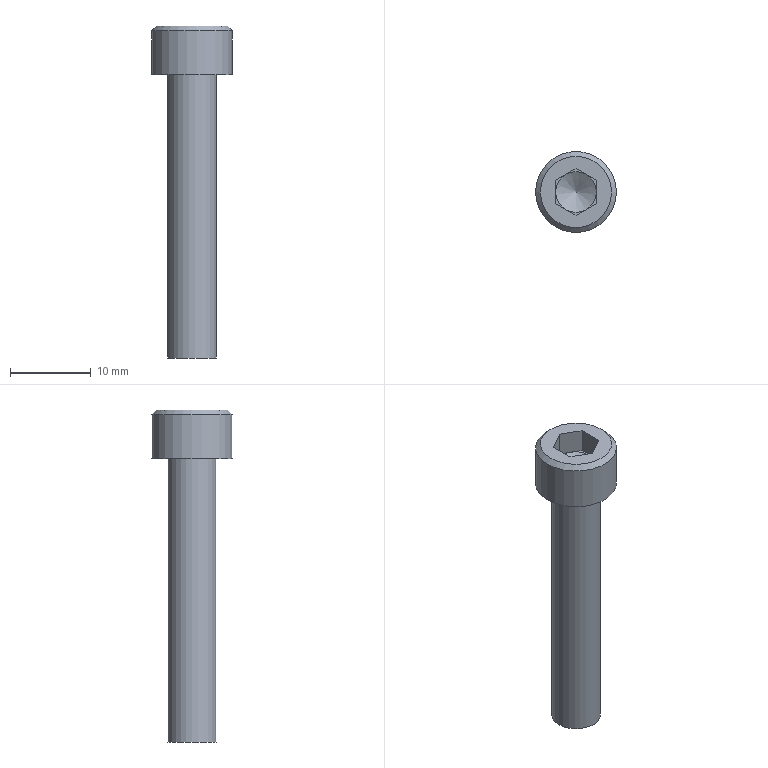Part | NX | features 5003_329_CB6-35 2 | 1 solid | 19 faces | box 10 x 10 x 41 mm | volume 1381 mm3 | plane 15 | cylinder 2 | cone 2 | commonest cylinder face diameters 6 x1 10 x1
STEP:
#1=CARTESIAN_POINT('',(55.2,-161.,-208.8));
#2=VERTEX_POINT('',#1);
#3=CARTESIAN_POINT('',(59.6,-161.,-208.8));
#4=DIRECTION('',(0.,0.,-1.));
#5=DIRECTION('',(-1.,0.,0.));
#6=AXIS2_PLACEMENT_3D('',#3,#4,#5);
#7=CIRCLE('',#6,4.4);
#8=EDGE_CURVE('',#2,#2,#7,.F.);
#9=ORIENTED_EDGE('',*,*,#8,.T.);
#10=EDGE_LOOP('',(#9));
#11=FACE_BOUND('',#10,.T.);
#12=CARTESIAN_POINT('',(59.6,-163.887,-208.8));
#13=VERTEX_POINT('',#12);
#14=CARTESIAN_POINT('',(62.1,-162.443,-208.8));
#15=VERTEX_POINT('',#14);
#16=CARTESIAN_POINT('',(59.6,-163.887,-208.8));
#17=DIRECTION('',(0.866,0.5,0.));
#18=VECTOR('',#17,1000.);
#19=LINE('',#16,#18);
#20=EDGE_CURVE('',#13,#15,#19,.T.);
#21=ORIENTED_EDGE('',*,*,#20,.F.);
#22=CARTESIAN_POINT('',(57.1,-162.443,-208.8));
#23=VERTEX_POINT('',#22);
#24=CARTESIAN_POINT('',(57.1,-162.443,-208.8));
#25=DIRECTION('',(0.866,-0.5,0.));
#26=VECTOR('',#25,1000.);
#27=LINE('',#24,#26);
#28=EDGE_CURVE('',#23,#13,#27,.T.);
#29=ORIENTED_EDGE('',*,*,#28,.F.);
#30=CARTESIAN_POINT('',(57.1,-159.557,-208.8));
#31=VERTEX_POINT('',#30);
#32=CARTESIAN_POINT('',(57.1,-159.557,-208.8));
#33=DIRECTION('',(0.,-1.,0.));
#34=VECTOR('',#33,1000.);
#35=LINE('',#32,#34);
#36=EDGE_CURVE('',#31,#23,#35,.T.);
#37=ORIENTED_EDGE('',*,*,#36,.F.);
#38=CARTESIAN_POINT('',(59.6,-158.113,-208.8));
#39=VERTEX_POINT('',#38);
#40=CARTESIAN_POINT('',(59.6,-158.113,-208.8));
#41=DIRECTION('',(-0.866,-0.5,0.));
#42=VECTOR('',#41,1000.);
#43=LINE('',#40,#42);
#44=EDGE_CURVE('',#39,#31,#43,.T.);
#45=ORIENTED_EDGE('',*,*,#44,.F.);
#46=CARTESIAN_POINT('',(62.1,-159.557,-208.8));
#47=VERTEX_POINT('',#46);
#48=CARTESIAN_POINT('',(62.1,-159.557,-208.8));
#49=DIRECTION('',(-0.866,0.5,0.));
#50=VECTOR('',#49,1000.);
#51=LINE('',#48,#50);
#52=EDGE_CURVE('',#47,#39,#51,.T.);
#53=ORIENTED_EDGE('',*,*,#52,.F.);
#54=CARTESIAN_POINT('',(62.1,-162.443,-208.8));
#55=DIRECTION('',(0.,1.,0.));
#56=VECTOR('',#55,1000.);
#57=LINE('',#54,#56);
#58=EDGE_CURVE('',#15,#47,#57,.T.);
#59=ORIENTED_EDGE('',*,*,#58,.F.);
#60=EDGE_LOOP('',(#21,#29,#37,#45,#53,#59));
#61=FACE_BOUND('',#60,.T.);
#62=CARTESIAN_POINT('',(59.6,-156.,-208.8));
#63=DIRECTION('',(0.,0.,-1.));
#64=DIRECTION('',(-1.,0.,0.));
#65=AXIS2_PLACEMENT_3D('',#62,#63,#64);
#66=PLANE('',#65);
#67=ADVANCED_FACE('',(#11,#61),#66,.F.);
#68=CARTESIAN_POINT('',(62.6,-161.,-249.8));
#69=VERTEX_POINT('',#68);
#70=CARTESIAN_POINT('',(59.6,-161.,-249.8));
#71=DIRECTION('',(0.,0.,1.));
#72=DIRECTION('',(1.,0.,0.));
#73=AXIS2_PLACEMENT_3D('',#70,#71,#72);
#74=CIRCLE('',#73,3.);
#75=EDGE_CURVE('',#69,#69,#74,.T.);
#76=ORIENTED_EDGE('',*,*,#75,.F.);
#77=EDGE_LOOP('',(#76));
#78=FACE_BOUND('',#77,.T.);
#79=CARTESIAN_POINT('',(59.6,-161.,-249.8));
#80=DIRECTION('',(0.,0.,1.));
#81=DIRECTION('',(1.,0.,0.));
#82=AXIS2_PLACEMENT_3D('',#79,#80,#81);
#83=PLANE('',#82);
#84=ADVANCED_FACE('',(#78),#83,.F.);
#85=CARTESIAN_POINT('',(62.6,-161.,-214.8));
#86=VERTEX_POINT('',#85);
#87=CARTESIAN_POINT('',(59.6,-161.,-214.8));
#88=DIRECTION('',(0.,0.,1.));
#89=DIRECTION('',(1.,0.,0.));
#90=AXIS2_PLACEMENT_3D('',#87,#88,#89);
#91=CIRCLE('',#90,3.);
#92=EDGE_CURVE('',#86,#86,#91,.T.);
#93=ORIENTED_EDGE('',*,*,#92,.F.);
#94=EDGE_LOOP('',(#93));
#95=FACE_BOUND('',#94,.T.);
#96=ORIENTED_EDGE('',*,*,#75,.T.);
#97=EDGE_LOOP('',(#96));
#98=FACE_BOUND('',#97,.T.);
#99=CARTESIAN_POINT('',(59.6,-161.,-208.8));
#100=DIRECTION('',(0.,0.,1.));
#101=DIRECTION('',(1.,0.,0.));
#102=AXIS2_PLACEMENT_3D('',#99,#100,#101);
#103=CYLINDRICAL_SURFACE('',#102,3.);
#104=ADVANCED_FACE('',(#95,#98),#103,.T.);
#105=CARTESIAN_POINT('',(64.6,-161.,-214.8));
#106=VERTEX_POINT('',#105);
#107=CARTESIAN_POINT('',(59.6,-161.,-214.8));
#108=DIRECTION('',(0.,0.,1.));
#109=DIRECTION('',(1.,0.,0.));
#110=AXIS2_PLACEMENT_3D('',#107,#108,#109);
#111=CIRCLE('',#110,5.);
#112=EDGE_CURVE('',#106,#106,#111,.T.);
#113=ORIENTED_EDGE('',*,*,#112,.F.);
#114=EDGE_LOOP('',(#113));
#115=FACE_BOUND('',#114,.T.);
#116=ORIENTED_EDGE('',*,*,#92,.T.);
#117=EDGE_LOOP('',(#116));
#118=FACE_BOUND('',#117,.T.);
#119=CARTESIAN_POINT('',(59.6,-158.,-214.8));
#120=DIRECTION('',(0.,0.,1.));
#121=DIRECTION('',(1.,0.,0.));
#122=AXIS2_PLACEMENT_3D('',#119,#120,#121);
#123=PLANE('',#122);
#124=ADVANCED_FACE('',(#115,#118),#123,.F.);
#125=CARTESIAN_POINT('',(54.6,-161.,-209.4));
#126=VERTEX_POINT('',#125);
#127=CARTESIAN_POINT('',(59.6,-161.,-209.4));
#128=DIRECTION('',(0.,0.,-1.));
#129=DIRECTION('',(-1.,0.,0.));
#130=AXIS2_PLACEMENT_3D('',#127,#128,#129);
#131=CIRCLE('',#130,5.);
#132=EDGE_CURVE('',#126,#126,#131,.T.);
#133=ORIENTED_EDGE('',*,*,#132,.T.);
#134=EDGE_LOOP('',(#133));
#135=FACE_BOUND('',#134,.T.);
#136=ORIENTED_EDGE('',*,*,#112,.T.);
#137=EDGE_LOOP('',(#136));
#138=FACE_BOUND('',#137,.T.);
#139=CARTESIAN_POINT('',(59.6,-161.,-208.8));
#140=DIRECTION('',(0.,0.,1.));
#141=DIRECTION('',(1.,0.,0.));
#142=AXIS2_PLACEMENT_3D('',#139,#140,#141);
#143=CYLINDRICAL_SURFACE('',#142,5.);
#144=ADVANCED_FACE('',(#135,#138),#143,.T.);
#145=ORIENTED_EDGE('',*,*,#132,.F.);
#146=EDGE_LOOP('',(#145));
#147=FACE_BOUND('',#146,.T.);
#148=ORIENTED_EDGE('',*,*,#8,.F.);
#149=EDGE_LOOP('',(#148));
#150=FACE_BOUND('',#149,.T.);
#151=CARTESIAN_POINT('',(59.6,-161.,-208.8));
#152=DIRECTION('',(0.,0.,-1.));
#153=DIRECTION('',(-1.,0.,0.));
#154=AXIS2_PLACEMENT_3D('',#151,#152,#153);
#155=CONICAL_SURFACE('',#154,4.4,0.7854);
#156=ADVANCED_FACE('',(#147,#150),#155,.T.);
#157=CARTESIAN_POINT('',(57.1,-162.443,-211.8));
#158=VERTEX_POINT('',#157);
#159=CARTESIAN_POINT('',(58.35,-163.165,-211.8));
#160=VERTEX_POINT('',#159);
#161=CARTESIAN_POINT('',(57.1,-162.443,-211.8));
#162=DIRECTION('',(0.866,-0.5,0.));
#163=VECTOR('',#162,1000.);
#164=LINE('',#161,#163);
#165=EDGE_CURVE('',#158,#160,#164,.T.);
#166=ORIENTED_EDGE('',*,*,#165,.F.);
#167=CARTESIAN_POINT('',(57.1,-162.443,-211.8));
#168=DIRECTION('',(0.,0.,1.));
#169=VECTOR('',#168,1000.);
#170=LINE('',#167,#169);
#171=EDGE_CURVE('',#158,#23,#170,.T.);
#172=ORIENTED_EDGE('',*,*,#171,.T.);
#173=ORIENTED_EDGE('',*,*,#28,.T.);
#174=CARTESIAN_POINT('',(59.6,-163.887,-211.8));
#175=VERTEX_POINT('',#174);
#176=CARTESIAN_POINT('',(59.6,-163.887,-211.8));
#177=DIRECTION('',(0.,0.,1.));
#178=VECTOR('',#177,1000.);
#179=LINE('',#176,#178);
#180=EDGE_CURVE('',#175,#13,#179,.T.);
#181=ORIENTED_EDGE('',*,*,#180,.F.);
#182=CARTESIAN_POINT('',(57.1,-162.443,-211.8));
#183=DIRECTION('',(0.866,-0.5,0.));
#184=VECTOR('',#183,1000.);
#185=LINE('',#182,#184);
#186=EDGE_CURVE('',#160,#175,#185,.T.);
#187=ORIENTED_EDGE('',*,*,#186,.F.);
#188=EDGE_LOOP('',(#166,#172,#173,#181,#187));
#189=FACE_BOUND('',#188,.T.);
#190=CARTESIAN_POINT('',(57.1,-162.443,-211.8));
#191=DIRECTION('',(-0.5,-0.866,0.));
#192=DIRECTION('',(-0.866,0.5,0.));
#193=AXIS2_PLACEMENT_3D('',#190,#191,#192);
#194=PLANE('',#193);
#195=ADVANCED_FACE('',(#189),#194,.F.);
#196=CARTESIAN_POINT('',(57.1,-159.557,-211.8));
#197=VERTEX_POINT('',#196);
#198=CARTESIAN_POINT('',(57.1,-161.,-211.8));
#199=VERTEX_POINT('',#198);
#200=CARTESIAN_POINT('',(57.1,-159.557,-211.8));
#201=DIRECTION('',(0.,-1.,0.));
#202=VECTOR('',#201,1000.);
#203=LINE('',#200,#202);
#204=EDGE_CURVE('',#197,#199,#203,.T.);
#205=ORIENTED_EDGE('',*,*,#204,.F.);
#206=CARTESIAN_POINT('',(57.1,-159.557,-211.8));
#207=DIRECTION('',(0.,0.,1.));
#208=VECTOR('',#207,1000.);
#209=LINE('',#206,#208);
#210=EDGE_CURVE('',#197,#31,#209,.T.);
#211=ORIENTED_EDGE('',*,*,#210,.T.);
#212=ORIENTED_EDGE('',*,*,#36,.T.);
#213=ORIENTED_EDGE('',*,*,#171,.F.);
#214=CARTESIAN_POINT('',(57.1,-159.557,-211.8));
#215=DIRECTION('',(0.,-1.,0.));
#216=VECTOR('',#215,1000.);
#217=LINE('',#214,#216);
#218=EDGE_CURVE('',#199,#158,#217,.T.);
#219=ORIENTED_EDGE('',*,*,#218,.F.);
#220=EDGE_LOOP('',(#205,#211,#212,#213,#219));
#221=FACE_BOUND('',#220,.T.);
#222=CARTESIAN_POINT('',(57.1,-159.557,-211.8));
#223=DIRECTION('',(-1.,0.,0.));
#224=DIRECTION('',(0.,1.,0.));
#225=AXIS2_PLACEMENT_3D('',#222,#223,#224);
#226=PLANE('',#225);
#227=ADVANCED_FACE('',(#221),#226,.F.);
#228=CARTESIAN_POINT('',(59.6,-158.113,-211.8));
#229=VERTEX_POINT('',#228);
#230=CARTESIAN_POINT('',(58.35,-158.835,-211.8));
#231=VERTEX_POINT('',#230);
#232=CARTESIAN_POINT('',(59.6,-158.113,-211.8));
#233=DIRECTION('',(-0.866,-0.5,0.));
#234=VECTOR('',#233,1000.);
#235=LINE('',#232,#234);
#236=EDGE_CURVE('',#229,#231,#235,.T.);
#237=ORIENTED_EDGE('',*,*,#236,.F.);
#238=CARTESIAN_POINT('',(59.6,-158.113,-211.8));
#239=DIRECTION('',(0.,0.,1.));
#240=VECTOR('',#239,1000.);
#241=LINE('',#238,#240);
#242=EDGE_CURVE('',#229,#39,#241,.T.);
#243=ORIENTED_EDGE('',*,*,#242,.T.);
#244=ORIENTED_EDGE('',*,*,#44,.T.);
#245=ORIENTED_EDGE('',*,*,#210,.F.);
#246=CARTESIAN_POINT('',(59.6,-158.113,-211.8));
#247=DIRECTION('',(-0.866,-0.5,0.));
#248=VECTOR('',#247,1000.);
#249=LINE('',#246,#248);
#250=EDGE_CURVE('',#231,#197,#249,.T.);
#251=ORIENTED_EDGE('',*,*,#250,.F.);
#252=EDGE_LOOP('',(#237,#243,#244,#245,#251));
#253=FACE_BOUND('',#252,.T.);
#254=CARTESIAN_POINT('',(59.6,-158.113,-211.8));
#255=DIRECTION('',(-0.5,0.866,0.));
#256=DIRECTION('',(0.866,0.5,0.));
#257=AXIS2_PLACEMENT_3D('',#254,#255,#256);
#258=PLANE('',#257);
#259=ADVANCED_FACE('',(#253),#258,.F.);
#260=CARTESIAN_POINT('',(62.1,-159.557,-211.8));
#261=VERTEX_POINT('',#260);
#262=CARTESIAN_POINT('',(60.85,-158.835,-211.8));
#263=VERTEX_POINT('',#262);
#264=CARTESIAN_POINT('',(62.1,-159.557,-211.8));
#265=DIRECTION('',(-0.866,0.5,0.));
#266=VECTOR('',#265,1000.);
#267=LINE('',#264,#266);
#268=EDGE_CURVE('',#261,#263,#267,.T.);
#269=ORIENTED_EDGE('',*,*,#268,.F.);
#270=CARTESIAN_POINT('',(62.1,-159.557,-211.8));
#271=DIRECTION('',(0.,0.,1.));
#272=VECTOR('',#271,1000.);
#273=LINE('',#270,#272);
#274=EDGE_CURVE('',#261,#47,#273,.T.);
#275=ORIENTED_EDGE('',*,*,#274,.T.);
#276=ORIENTED_EDGE('',*,*,#52,.T.);
#277=ORIENTED_EDGE('',*,*,#242,.F.);
#278=CARTESIAN_POINT('',(62.1,-159.557,-211.8));
#279=DIRECTION('',(-0.866,0.5,0.));
#280=VECTOR('',#279,1000.);
#281=LINE('',#278,#280);
#282=EDGE_CURVE('',#263,#229,#281,.T.);
#283=ORIENTED_EDGE('',*,*,#282,.F.);
#284=EDGE_LOOP('',(#269,#275,#276,#277,#283));
#285=FACE_BOUND('',#284,.T.);
#286=CARTESIAN_POINT('',(62.1,-159.557,-211.8));
#287=DIRECTION('',(0.5,0.866,0.));
#288=DIRECTION('',(0.866,-0.5,0.));
#289=AXIS2_PLACEMENT_3D('',#286,#287,#288);
#290=PLANE('',#289);
#291=ADVANCED_FACE('',(#285),#290,.F.);
#292=CARTESIAN_POINT('',(62.1,-162.443,-211.8));
#293=VERTEX_POINT('',#292);
#294=CARTESIAN_POINT('',(62.1,-161.,-211.8));
#295=VERTEX_POINT('',#294);
#296=CARTESIAN_POINT('',(62.1,-162.443,-211.8));
#297=DIRECTION('',(0.,1.,0.));
#298=VECTOR('',#297,1000.);
#299=LINE('',#296,#298);
#300=EDGE_CURVE('',#293,#295,#299,.T.);
#301=ORIENTED_EDGE('',*,*,#300,.F.);
#302=CARTESIAN_POINT('',(62.1,-162.443,-211.8));
#303=DIRECTION('',(0.,0.,1.));
#304=VECTOR('',#303,1000.);
#305=LINE('',#302,#304);
#306=EDGE_CURVE('',#293,#15,#305,.T.);
#307=ORIENTED_EDGE('',*,*,#306,.T.);
#308=ORIENTED_EDGE('',*,*,#58,.T.);
#309=ORIENTED_EDGE('',*,*,#274,.F.);
#310=CARTESIAN_POINT('',(62.1,-162.443,-211.8));
#311=DIRECTION('',(0.,1.,0.));
#312=VECTOR('',#311,1000.);
#313=LINE('',#310,#312);
#314=EDGE_CURVE('',#295,#261,#313,.T.);
#315=ORIENTED_EDGE('',*,*,#314,.F.);
#316=EDGE_LOOP('',(#301,#307,#308,#309,#315));
#317=FACE_BOUND('',#316,.T.);
#318=CARTESIAN_POINT('',(62.1,-162.443,-211.8));
#319=DIRECTION('',(1.,0.,0.));
#320=DIRECTION('',(0.,0.,-1.));
#321=AXIS2_PLACEMENT_3D('',#318,#319,#320);
#322=PLANE('',#321);
#323=ADVANCED_FACE('',(#317),#322,.F.);
#324=CARTESIAN_POINT('',(60.85,-163.165,-211.8));
#325=VERTEX_POINT('',#324);
#326=CARTESIAN_POINT('',(59.6,-163.887,-211.8));
#327=DIRECTION('',(0.866,0.5,0.));
#328=VECTOR('',#327,1000.);
#329=LINE('',#326,#328);
#330=EDGE_CURVE('',#175,#325,#329,.T.);
#331=ORIENTED_EDGE('',*,*,#330,.F.);
#332=ORIENTED_EDGE('',*,*,#180,.T.);
#333=ORIENTED_EDGE('',*,*,#20,.T.);
#334=ORIENTED_EDGE('',*,*,#306,.F.);
#335=CARTESIAN_POINT('',(59.6,-163.887,-211.8));
#336=DIRECTION('',(0.866,0.5,0.));
#337=VECTOR('',#336,1000.);
#338=LINE('',#335,#337);
#339=EDGE_CURVE('',#325,#293,#338,.T.);
#340=ORIENTED_EDGE('',*,*,#339,.F.);
#341=EDGE_LOOP('',(#331,#332,#333,#334,#340));
#342=FACE_BOUND('',#341,.T.);
#343=CARTESIAN_POINT('',(59.6,-163.887,-211.8));
#344=DIRECTION('',(0.5,-0.866,0.));
#345=DIRECTION('',(-0.866,-0.5,0.));
#346=AXIS2_PLACEMENT_3D('',#343,#344,#345);
#347=PLANE('',#346);
#348=ADVANCED_FACE('',(#342),#347,.F.);
#349=ORIENTED_EDGE('',*,*,#314,.T.);
#350=ORIENTED_EDGE('',*,*,#268,.T.);
#351=CARTESIAN_POINT('',(59.6,-161.,-211.8));
#352=DIRECTION('',(0.,0.,1.));
#353=DIRECTION('',(0.,-1.,0.));
#354=AXIS2_PLACEMENT_3D('',#351,#352,#353);
#355=CIRCLE('',#354,2.5);
#356=EDGE_CURVE('',#295,#263,#355,.T.);
#357=ORIENTED_EDGE('',*,*,#356,.F.);
#358=EDGE_LOOP('',(#349,#350,#357));
#359=FACE_BOUND('',#358,.T.);
#360=CARTESIAN_POINT('',(59.6,-161.,-211.8));
#361=DIRECTION('',(0.,0.,1.));
#362=DIRECTION('',(1.,0.,0.));
#363=AXIS2_PLACEMENT_3D('',#360,#361,#362);
#364=PLANE('',#363);
#365=ADVANCED_FACE('',(#359),#364,.T.);
#366=ORIENTED_EDGE('',*,*,#282,.T.);
#367=ORIENTED_EDGE('',*,*,#236,.T.);
#368=CARTESIAN_POINT('',(59.6,-161.,-211.8));
#369=DIRECTION('',(0.,0.,1.));
#370=DIRECTION('',(0.,-1.,0.));
#371=AXIS2_PLACEMENT_3D('',#368,#369,#370);
#372=CIRCLE('',#371,2.5);
#373=EDGE_CURVE('',#263,#231,#372,.T.);
#374=ORIENTED_EDGE('',*,*,#373,.F.);
#375=EDGE_LOOP('',(#366,#367,#374));
#376=FACE_BOUND('',#375,.T.);
#377=CARTESIAN_POINT('',(59.6,-161.,-211.8));
#378=DIRECTION('',(0.,0.,1.));
#379=DIRECTION('',(1.,0.,0.));
#380=AXIS2_PLACEMENT_3D('',#377,#378,#379);
#381=PLANE('',#380);
#382=ADVANCED_FACE('',(#376),#381,.T.);
#383=ORIENTED_EDGE('',*,*,#250,.T.);
#384=ORIENTED_EDGE('',*,*,#204,.T.);
#385=CARTESIAN_POINT('',(59.6,-161.,-211.8));
#386=DIRECTION('',(0.,0.,1.));
#387=DIRECTION('',(0.,-1.,0.));
#388=AXIS2_PLACEMENT_3D('',#385,#386,#387);
#389=CIRCLE('',#388,2.5);
#390=EDGE_CURVE('',#231,#199,#389,.T.);
#391=ORIENTED_EDGE('',*,*,#390,.F.);
#392=EDGE_LOOP('',(#383,#384,#391));
#393=FACE_BOUND('',#392,.T.);
#394=CARTESIAN_POINT('',(59.6,-161.,-211.8));
#395=DIRECTION('',(0.,0.,1.));
#396=DIRECTION('',(1.,0.,0.));
#397=AXIS2_PLACEMENT_3D('',#394,#395,#396);
#398=PLANE('',#397);
#399=ADVANCED_FACE('',(#393),#398,.T.);
#400=ORIENTED_EDGE('',*,*,#218,.T.);
#401=ORIENTED_EDGE('',*,*,#165,.T.);
#402=CARTESIAN_POINT('',(59.6,-161.,-211.8));
#403=DIRECTION('',(0.,0.,1.));
#404=DIRECTION('',(0.,-1.,0.));
#405=AXIS2_PLACEMENT_3D('',#402,#403,#404);
#406=CIRCLE('',#405,2.5);
#407=EDGE_CURVE('',#199,#160,#406,.T.);
#408=ORIENTED_EDGE('',*,*,#407,.F.);
#409=EDGE_LOOP('',(#400,#401,#408));
#410=FACE_BOUND('',#409,.T.);
#411=CARTESIAN_POINT('',(59.6,-161.,-211.8));
#412=DIRECTION('',(0.,0.,1.));
#413=DIRECTION('',(1.,0.,0.));
#414=AXIS2_PLACEMENT_3D('',#411,#412,#413);
#415=PLANE('',#414);
#416=ADVANCED_FACE('',(#410),#415,.T.);
#417=ORIENTED_EDGE('',*,*,#186,.T.);
#418=ORIENTED_EDGE('',*,*,#330,.T.);
#419=CARTESIAN_POINT('',(59.6,-161.,-211.8));
#420=DIRECTION('',(0.,0.,1.));
#421=DIRECTION('',(0.,-1.,0.));
#422=AXIS2_PLACEMENT_3D('',#419,#420,#421);
#423=CIRCLE('',#422,2.5);
#424=EDGE_CURVE('',#160,#325,#423,.T.);
#425=ORIENTED_EDGE('',*,*,#424,.F.);
#426=EDGE_LOOP('',(#417,#418,#425));
#427=FACE_BOUND('',#426,.T.);
#428=CARTESIAN_POINT('',(59.6,-161.,-211.8));
#429=DIRECTION('',(0.,0.,1.));
#430=DIRECTION('',(1.,0.,0.));
#431=AXIS2_PLACEMENT_3D('',#428,#429,#430);
#432=PLANE('',#431);
#433=ADVANCED_FACE('',(#427),#432,.T.);
#434=ORIENTED_EDGE('',*,*,#339,.T.);
#435=ORIENTED_EDGE('',*,*,#300,.T.);
#436=CARTESIAN_POINT('',(59.6,-161.,-211.8));
#437=DIRECTION('',(0.,0.,1.));
#438=DIRECTION('',(0.,-1.,0.));
#439=AXIS2_PLACEMENT_3D('',#436,#437,#438);
#440=CIRCLE('',#439,2.5);
#441=EDGE_CURVE('',#325,#295,#440,.T.);
#442=ORIENTED_EDGE('',*,*,#441,.F.);
#443=EDGE_LOOP('',(#434,#435,#442));
#444=FACE_BOUND('',#443,.T.);
#445=CARTESIAN_POINT('',(59.6,-161.,-211.8));
#446=DIRECTION('',(0.,0.,1.));
#447=DIRECTION('',(1.,0.,0.));
#448=AXIS2_PLACEMENT_3D('',#445,#446,#447);
#449=PLANE('',#448);
#450=ADVANCED_FACE('',(#444),#449,.T.);
#451=ORIENTED_EDGE('',*,*,#441,.T.);
#452=ORIENTED_EDGE('',*,*,#356,.T.);
#453=ORIENTED_EDGE('',*,*,#373,.T.);
#454=ORIENTED_EDGE('',*,*,#390,.T.);
#455=ORIENTED_EDGE('',*,*,#407,.T.);
#456=ORIENTED_EDGE('',*,*,#424,.T.);
#457=EDGE_LOOP('',(#451,#452,#453,#454,#455,#456));
#458=FACE_BOUND('',#457,.T.);
#459=CARTESIAN_POINT('',(59.6,-161.,-213.302));
#460=VERTEX_POINT('',#459);
#461=VERTEX_LOOP('',#460);
#462=FACE_BOUND('',#461,.T.);
#463=CARTESIAN_POINT('',(59.6,-161.,-213.302));
#464=DIRECTION('',(0.,0.,1.));
#465=DIRECTION('',(0.,-1.,0.));
#466=AXIS2_PLACEMENT_3D('',#463,#464,#465);
#467=CONICAL_SURFACE('',#466,0.,1.03);
#468=ADVANCED_FACE('',(#458,#462),#467,.F.);
#469=CLOSED_SHELL('',(#67,#84,#104,#124,#144,#156,#195,#227,#259,#291,#323,#348,#365,#382,#399,#416,#433,#450,#468));
#470=MANIFOLD_SOLID_BREP('',#469);
#471=(LENGTH_UNIT()NAMED_UNIT(*)SI_UNIT(.MILLI.,.METRE.));
#472=UNCERTAINTY_MEASURE_WITH_UNIT(LENGTH_MEASURE(0.00001),#471,'','');
#473=(NAMED_UNIT(*)PLANE_ANGLE_UNIT()SI_UNIT($,.RADIAN.));
#474=(NAMED_UNIT(*)SI_UNIT($,.STERADIAN.)SOLID_ANGLE_UNIT());
#475=(GEOMETRIC_REPRESENTATION_CONTEXT(3)GLOBAL_UNCERTAINTY_ASSIGNED_CONTEXT((#472))GLOBAL_UNIT_ASSIGNED_CONTEXT((#471,#473,#474))REPRESENTATION_CONTEXT('',''));
#476=ADVANCED_BREP_SHAPE_REPRESENTATION('',(#470),#475);